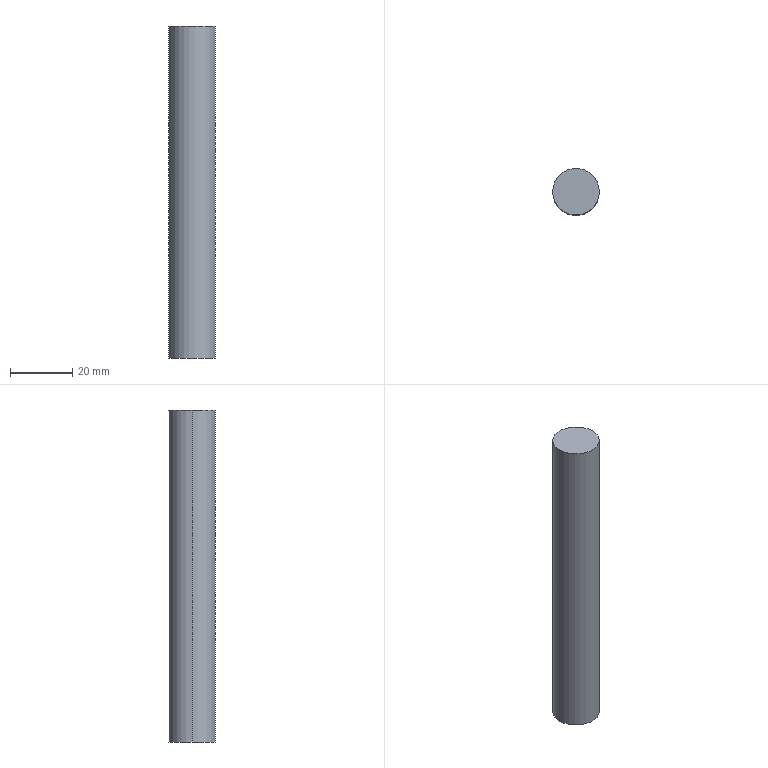Part | SolidWorks | features Extrusion 1 | 1 solid | 4 faces | box 15 x 15 x 107 mm | volume 18908 mm3 | cylinder 2 | plane 2 | commonest cylinder face diameters 15 x2
STEP:
#1=CARTESIAN_POINT('',(7.5,0.,-13.));
#2=VERTEX_POINT('',#1);
#3=CARTESIAN_POINT('',(-7.5,0.,-13.));
#4=VERTEX_POINT('',#3);
#5=CARTESIAN_POINT('',(0.,0.,-13.));
#6=DIRECTION('',(0.,0.,1.));
#7=DIRECTION('',(1.,0.,0.));
#8=AXIS2_PLACEMENT_3D('',#5,#6,#7);
#9=CIRCLE('',#8,7.5);
#10=EDGE_CURVE('',#2,#4,#9,.T.);
#11=ORIENTED_EDGE('',*,*,#10,.T.);
#12=CARTESIAN_POINT('',(-7.5,0.,94.));
#13=VERTEX_POINT('',#12);
#14=CARTESIAN_POINT('',(-7.5,0.,-13.));
#15=DIRECTION('',(0.,0.,1.));
#16=VECTOR('',#15,1000.);
#17=LINE('',#14,#16);
#18=EDGE_CURVE('',#4,#13,#17,.T.);
#19=ORIENTED_EDGE('',*,*,#18,.T.);
#20=CARTESIAN_POINT('',(7.5,0.,94.));
#21=VERTEX_POINT('',#20);
#22=CARTESIAN_POINT('',(0.,0.,94.));
#23=DIRECTION('',(0.,0.,1.));
#24=DIRECTION('',(1.,0.,0.));
#25=AXIS2_PLACEMENT_3D('',#22,#23,#24);
#26=CIRCLE('',#25,7.5);
#27=EDGE_CURVE('',#21,#13,#26,.T.);
#28=ORIENTED_EDGE('',*,*,#27,.F.);
#29=CARTESIAN_POINT('',(7.5,0.,-13.));
#30=DIRECTION('',(0.,0.,1.));
#31=VECTOR('',#30,1000.);
#32=LINE('',#29,#31);
#33=EDGE_CURVE('',#2,#21,#32,.T.);
#34=ORIENTED_EDGE('',*,*,#33,.F.);
#35=EDGE_LOOP('',(#11,#19,#28,#34));
#36=FACE_OUTER_BOUND('',#35,.T.);
#37=CARTESIAN_POINT('',(0.,0.,-13.));
#38=DIRECTION('',(0.,0.,1.));
#39=DIRECTION('',(1.,0.,0.));
#40=AXIS2_PLACEMENT_3D('',#37,#38,#39);
#41=CYLINDRICAL_SURFACE('',#40,7.5);
#42=ADVANCED_FACE('',(#36),#41,.T.);
#43=ORIENTED_EDGE('',*,*,#18,.F.);
#44=CARTESIAN_POINT('',(0.,0.,-13.));
#45=DIRECTION('',(0.,0.,1.));
#46=DIRECTION('',(1.,0.,0.));
#47=AXIS2_PLACEMENT_3D('',#44,#45,#46);
#48=CIRCLE('',#47,7.5);
#49=EDGE_CURVE('',#4,#2,#48,.T.);
#50=ORIENTED_EDGE('',*,*,#49,.T.);
#51=ORIENTED_EDGE('',*,*,#33,.T.);
#52=CARTESIAN_POINT('',(0.,0.,94.));
#53=DIRECTION('',(0.,0.,1.));
#54=DIRECTION('',(1.,0.,0.));
#55=AXIS2_PLACEMENT_3D('',#52,#53,#54);
#56=CIRCLE('',#55,7.5);
#57=EDGE_CURVE('',#13,#21,#56,.T.);
#58=ORIENTED_EDGE('',*,*,#57,.F.);
#59=EDGE_LOOP('',(#43,#50,#51,#58));
#60=FACE_OUTER_BOUND('',#59,.T.);
#61=CARTESIAN_POINT('',(0.,0.,-13.));
#62=DIRECTION('',(0.,0.,1.));
#63=DIRECTION('',(1.,0.,0.));
#64=AXIS2_PLACEMENT_3D('',#61,#62,#63);
#65=CYLINDRICAL_SURFACE('',#64,7.5);
#66=ADVANCED_FACE('',(#60),#65,.T.);
#67=ORIENTED_EDGE('',*,*,#10,.F.);
#68=ORIENTED_EDGE('',*,*,#49,.F.);
#69=EDGE_LOOP('',(#67,#68));
#70=FACE_OUTER_BOUND('',#69,.T.);
#71=CARTESIAN_POINT('',(0.,0.,-13.));
#72=DIRECTION('',(0.,0.,1.));
#73=DIRECTION('',(1.,0.,0.));
#74=AXIS2_PLACEMENT_3D('',#71,#72,#73);
#75=PLANE('',#74);
#76=ADVANCED_FACE('',(#70),#75,.F.);
#77=ORIENTED_EDGE('',*,*,#27,.T.);
#78=ORIENTED_EDGE('',*,*,#57,.T.);
#79=EDGE_LOOP('',(#77,#78));
#80=FACE_OUTER_BOUND('',#79,.T.);
#81=CARTESIAN_POINT('',(0.,0.,94.));
#82=DIRECTION('',(0.,0.,1.));
#83=DIRECTION('',(1.,0.,0.));
#84=AXIS2_PLACEMENT_3D('',#81,#82,#83);
#85=PLANE('',#84);
#86=ADVANCED_FACE('',(#80),#85,.T.);
#87=CLOSED_SHELL('',(#42,#66,#76,#86));
#88=MANIFOLD_SOLID_BREP('',#87);
#89=CARTESIAN_POINT('',(0.,0.,0.));
#90=DIRECTION('',(0.,0.,1.));
#91=DIRECTION('',(1.,0.,0.));
#92=AXIS2_PLACEMENT_3D('',#89,#90,#91);
#93=(LENGTH_UNIT()NAMED_UNIT(*)SI_UNIT(.MILLI.,.METRE.));
#94=UNCERTAINTY_MEASURE_WITH_UNIT(LENGTH_MEASURE(0.00001),#93,'','');
#95=(NAMED_UNIT(*)PLANE_ANGLE_UNIT()SI_UNIT($,.RADIAN.));
#96=(NAMED_UNIT(*)SI_UNIT($,.STERADIAN.)SOLID_ANGLE_UNIT());
#97=(GEOMETRIC_REPRESENTATION_CONTEXT(3)GLOBAL_UNCERTAINTY_ASSIGNED_CONTEXT((#94))GLOBAL_UNIT_ASSIGNED_CONTEXT((#93,#95,#96))REPRESENTATION_CONTEXT('',''));
#98=ADVANCED_BREP_SHAPE_REPRESENTATION('',(#88,#92),#97);